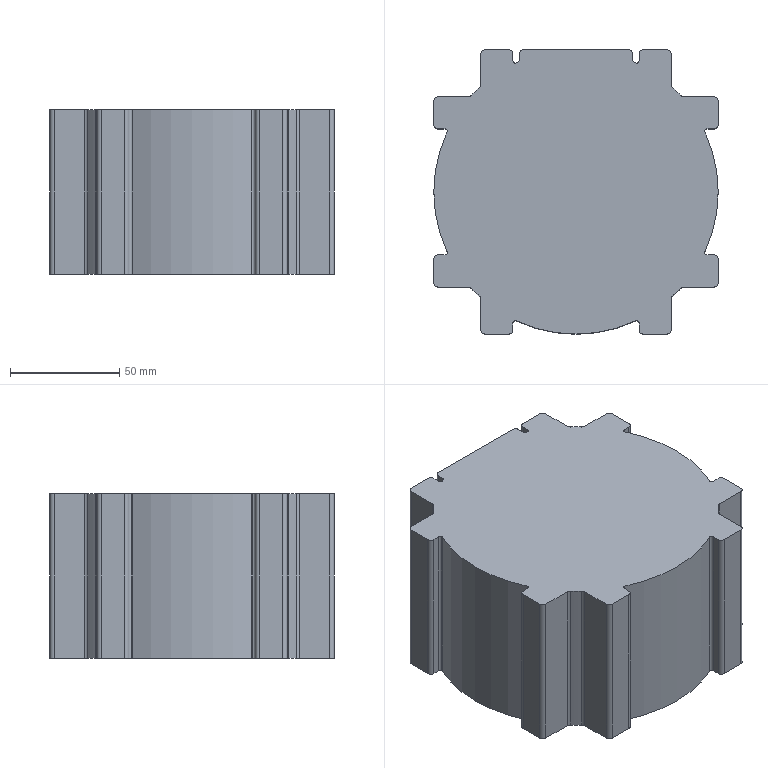Part | STEP file | 31090369--ISMH3-850001 | 1 solid | 80 faces | box 130 x 130 x 75 mm | volume 1096871 mm3 | cylinder 50 | plane 30 | commonest cylinder face diameters 4 x26 2 x12 130 x10 22 x2